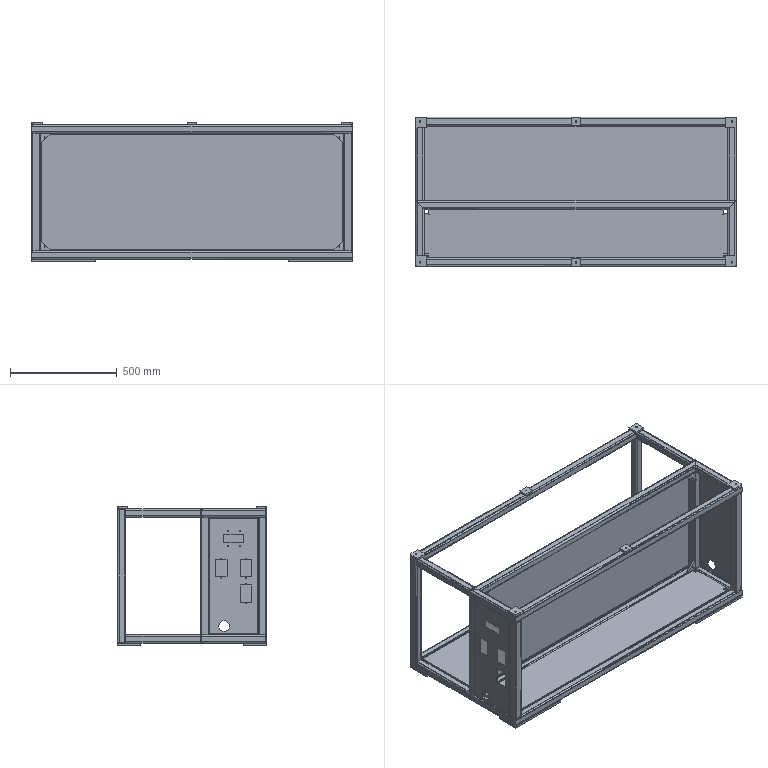Part | STEP file | QA-机箱-1(Default_As Machined_) | 47 solids | 640 faces | box 1500 x 700 x 650 mm | volume 12485783 mm3 | plane 382 | cylinder 258 | commonest cylinder face diameters 8 x72 16 x64 6.8 x26 10 x20 2 x16 6 x16